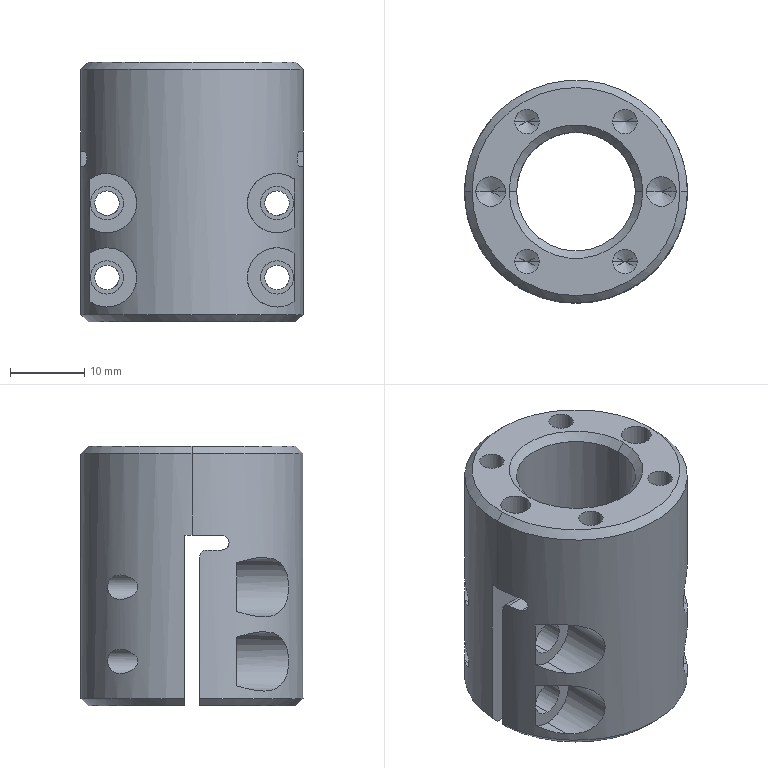Part | STEP file | 11-FG-SB00211 | 1 solid | 85 faces | box 30 x 30 x 35 mm | volume 14894 mm3 | cylinder 50 | cone 20 | plane 15 | commonest cylinder face diameters 3.3 x16 8 x12 4.5 x8 2 x6 4 x4 16 x2